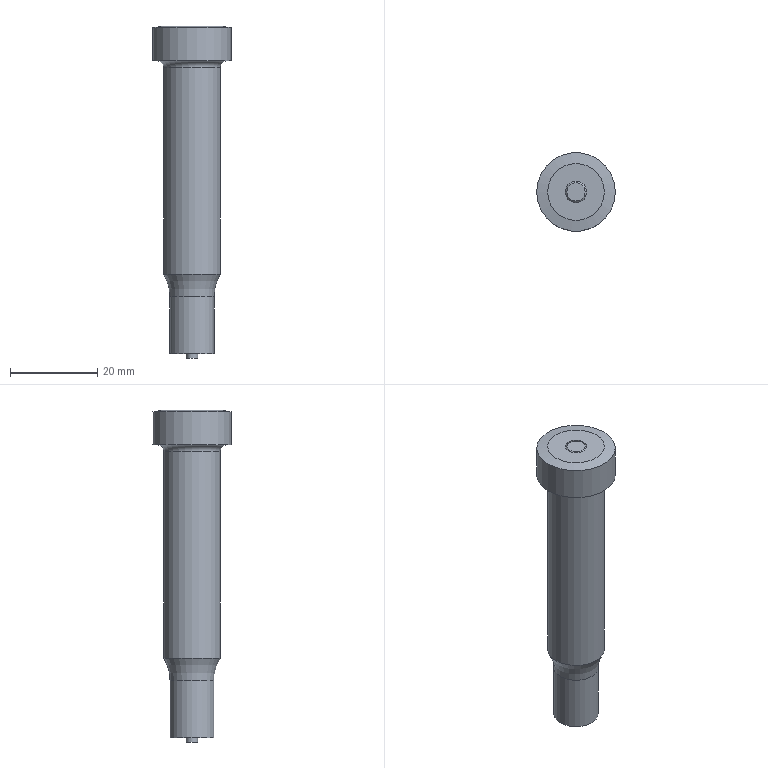Part | NX | features APJAS13-90-P10.10_2 2 | 1 solid | 20 faces | box 18 x 18 x 76 mm | volume 9972 mm3 | cylinder 8 | plane 7 | torus 2 | cone 2 | spline 1 | commonest cylinder face diameters 2.6 x1 2.8 x1 4.2 x1 4.4 x1 4.9 x1 10.1 x1
STEP:
#1=CARTESIAN_POINT('',(-223.5,0.,13.186));
#2=VERTEX_POINT('',#1);
#3=CARTESIAN_POINT('',(-230.,0.,13.186));
#4=DIRECTION('',(0.,0.,1.));
#5=DIRECTION('',(-1.,0.,0.));
#6=AXIS2_PLACEMENT_3D('',#3,#4,#5);
#7=CIRCLE('',#6,6.5);
#8=EDGE_CURVE('',#2,#2,#7,.T.);
#9=ORIENTED_EDGE('',*,*,#8,.T.);
#10=EDGE_LOOP('',(#9));
#11=FACE_BOUND('',#10,.T.);
#12=CARTESIAN_POINT('',(-236.5,0.,60.5));
#13=VERTEX_POINT('',#12);
#14=CARTESIAN_POINT('',(-230.,0.,60.5));
#15=DIRECTION('',(0.,0.,1.));
#16=DIRECTION('',(1.,0.,0.));
#17=AXIS2_PLACEMENT_3D('',#14,#15,#16);
#18=CIRCLE('',#17,6.5);
#19=EDGE_CURVE('',#13,#13,#18,.T.);
#20=ORIENTED_EDGE('',*,*,#19,.F.);
#21=EDGE_LOOP('',(#20));
#22=FACE_BOUND('',#21,.T.);
#23=CARTESIAN_POINT('',(-230.,0.,42.5));
#24=DIRECTION('',(0.,0.,-1.));
#25=DIRECTION('',(1.,0.,0.));
#26=AXIS2_PLACEMENT_3D('',#23,#24,#25);
#27=CYLINDRICAL_SURFACE('',#26,6.5);
#28=ADVANCED_FACE('',(#11,#22),#27,.T.);
#29=CARTESIAN_POINT('',(-231.4,0.,23.));
#30=VERTEX_POINT('',#29);
#31=CARTESIAN_POINT('',(-230.,0.,23.));
#32=DIRECTION('',(0.,0.,1.));
#33=DIRECTION('',(-1.,0.,0.));
#34=AXIS2_PLACEMENT_3D('',#31,#32,#33);
#35=CIRCLE('',#34,1.4);
#36=EDGE_CURVE('',#30,#30,#35,.T.);
#37=ORIENTED_EDGE('',*,*,#36,.T.);
#38=EDGE_LOOP('',(#37));
#39=FACE_BOUND('',#38,.T.);
#40=CARTESIAN_POINT('',(-231.4,0.,-5.));
#41=VERTEX_POINT('',#40);
#42=CARTESIAN_POINT('',(-230.,0.,-5.));
#43=DIRECTION('',(0.,0.,1.));
#44=DIRECTION('',(-1.,0.,0.));
#45=AXIS2_PLACEMENT_3D('',#42,#43,#44);
#46=CIRCLE('',#45,1.4);
#47=EDGE_CURVE('',#41,#41,#46,.T.);
#48=ORIENTED_EDGE('',*,*,#47,.F.);
#49=EDGE_LOOP('',(#48));
#50=FACE_BOUND('',#49,.T.);
#51=CARTESIAN_POINT('',(-230.,0.,9.));
#52=DIRECTION('',(0.,0.,-1.));
#53=DIRECTION('',(1.,0.,0.));
#54=AXIS2_PLACEMENT_3D('',#51,#52,#53);
#55=CYLINDRICAL_SURFACE('',#54,1.4);
#56=ADVANCED_FACE('',(#39,#50),#55,.F.);
#57=CARTESIAN_POINT('',(-227.55,0.,69.632));
#58=VERTEX_POINT('',#57);
#59=CARTESIAN_POINT('',(-230.,0.,69.632));
#60=DIRECTION('',(0.,0.,1.));
#61=DIRECTION('',(1.,0.,0.));
#62=AXIS2_PLACEMENT_3D('',#59,#60,#61);
#63=CIRCLE('',#62,2.45);
#64=EDGE_CURVE('',#58,#58,#63,.T.);
#65=ORIENTED_EDGE('',*,*,#64,.F.);
#66=EDGE_LOOP('',(#65));
#67=FACE_BOUND('',#66,.T.);
#68=CARTESIAN_POINT('',(-232.45,0.,70.));
#69=VERTEX_POINT('',#68);
#70=CARTESIAN_POINT('',(-230.,0.,70.));
#71=DIRECTION('',(0.,0.,-1.));
#72=DIRECTION('',(-1.,0.,0.));
#73=AXIS2_PLACEMENT_3D('',#70,#71,#72);
#74=CIRCLE('',#73,2.45);
#75=EDGE_CURVE('',#69,#69,#74,.T.);
#76=ORIENTED_EDGE('',*,*,#75,.F.);
#77=EDGE_LOOP('',(#76));
#78=FACE_BOUND('',#77,.T.);
#79=CARTESIAN_POINT('',(-230.,0.,68.775));
#80=DIRECTION('',(0.,0.,-1.));
#81=DIRECTION('',(1.,0.,0.));
#82=AXIS2_PLACEMENT_3D('',#79,#80,#81);
#83=CYLINDRICAL_SURFACE('',#82,2.45);
#84=ADVANCED_FACE('',(#67,#78),#83,.F.);
#85=ORIENTED_EDGE('',*,*,#19,.T.);
#86=EDGE_LOOP('',(#85));
#87=FACE_BOUND('',#86,.T.);
#88=CARTESIAN_POINT('',(-238.,0.,62.));
#89=VERTEX_POINT('',#88);
#90=CARTESIAN_POINT('',(-230.,0.,62.));
#91=DIRECTION('',(0.,0.,-1.));
#92=DIRECTION('',(1.,0.,0.));
#93=AXIS2_PLACEMENT_3D('',#90,#91,#92);
#94=CIRCLE('',#93,8.);
#95=EDGE_CURVE('',#89,#89,#94,.T.);
#96=ORIENTED_EDGE('',*,*,#95,.T.);
#97=EDGE_LOOP('',(#96));
#98=FACE_BOUND('',#97,.T.);
#99=CARTESIAN_POINT('',(-230.,0.,60.5));
#100=DIRECTION('',(0.,0.,1.));
#101=DIRECTION('',(-1.,0.,0.));
#102=AXIS2_PLACEMENT_3D('',#99,#100,#101);
#103=TOROIDAL_SURFACE('',#102,8.,1.5);
#104=ADVANCED_FACE('',(#87,#98),#103,.F.);
#105=CARTESIAN_POINT('',(-239.,0.,62.));
#106=VERTEX_POINT('',#105);
#107=CARTESIAN_POINT('',(-230.,0.,62.));
#108=DIRECTION('',(0.,0.,-1.));
#109=DIRECTION('',(-1.,0.,0.));
#110=AXIS2_PLACEMENT_3D('',#107,#108,#109);
#111=CIRCLE('',#110,9.);
#112=EDGE_CURVE('',#106,#106,#111,.T.);
#113=ORIENTED_EDGE('',*,*,#112,.T.);
#114=EDGE_LOOP('',(#113));
#115=FACE_BOUND('',#114,.T.);
#116=ORIENTED_EDGE('',*,*,#95,.F.);
#117=EDGE_LOOP('',(#116));
#118=FACE_BOUND('',#117,.T.);
#119=CARTESIAN_POINT('',(-230.,0.,62.));
#120=DIRECTION('',(0.,0.,-1.));
#121=DIRECTION('',(1.,0.,0.));
#122=AXIS2_PLACEMENT_3D('',#119,#120,#121);
#123=PLANE('',#122);
#124=ADVANCED_FACE('',(#115,#118),#123,.T.);
#125=CARTESIAN_POINT('',(-235.05,0.,8.));
#126=VERTEX_POINT('',#125);
#127=CARTESIAN_POINT('',(-230.,0.,8.));
#128=DIRECTION('',(0.,0.,1.));
#129=DIRECTION('',(-1.,0.,0.));
#130=AXIS2_PLACEMENT_3D('',#127,#128,#129);
#131=CIRCLE('',#130,5.05);
#132=EDGE_CURVE('',#126,#126,#131,.T.);
#133=ORIENTED_EDGE('',*,*,#132,.T.);
#134=EDGE_LOOP('',(#133));
#135=FACE_BOUND('',#134,.T.);
#136=ORIENTED_EDGE('',*,*,#8,.F.);
#137=EDGE_LOOP('',(#136));
#138=FACE_BOUND('',#137,.T.);
#139=CARTESIAN_POINT('',(-230.,0.,8.));
#140=DIRECTION('',(0.,0.,-1.));
#141=DIRECTION('',(1.,0.,0.));
#142=AXIS2_PLACEMENT_3D('',#139,#140,#141);
#143=TOROIDAL_SURFACE('',#142,15.05,10.);
#144=ADVANCED_FACE('',(#135,#138),#143,.F.);
#145=CARTESIAN_POINT('',(-239.,0.,69.559));
#146=VERTEX_POINT('',#145);
#147=CARTESIAN_POINT('',(-230.,0.,69.559));
#148=DIRECTION('',(0.,0.,1.));
#149=DIRECTION('',(1.,0.,0.));
#150=AXIS2_PLACEMENT_3D('',#147,#148,#149);
#151=CIRCLE('',#150,9.);
#152=EDGE_CURVE('',#146,#146,#151,.T.);
#153=ORIENTED_EDGE('',*,*,#152,.T.);
#154=EDGE_LOOP('',(#153));
#155=FACE_BOUND('',#154,.T.);
#156=CARTESIAN_POINT('',(-236.5,0.,70.));
#157=VERTEX_POINT('',#156);
#158=CARTESIAN_POINT('',(-230.,0.,70.));
#159=DIRECTION('',(0.,0.,-1.));
#160=DIRECTION('',(1.,0.,0.));
#161=AXIS2_PLACEMENT_3D('',#158,#159,#160);
#162=CIRCLE('',#161,6.5);
#163=EDGE_CURVE('',#157,#157,#162,.T.);
#164=ORIENTED_EDGE('',*,*,#163,.T.);
#165=EDGE_LOOP('',(#164));
#166=FACE_BOUND('',#165,.T.);
#167=CARTESIAN_POINT('',(-230.,0.,70.));
#168=DIRECTION('',(0.,0.,-1.));
#169=DIRECTION('',(-1.,0.,0.));
#170=AXIS2_PLACEMENT_3D('',#167,#168,#169);
#171=CONICAL_SURFACE('',#170,6.5,1.396);
#172=ADVANCED_FACE('',(#155,#166),#171,.T.);
#173=ORIENTED_EDGE('',*,*,#112,.F.);
#174=EDGE_LOOP('',(#173));
#175=FACE_BOUND('',#174,.T.);
#176=ORIENTED_EDGE('',*,*,#152,.F.);
#177=EDGE_LOOP('',(#176));
#178=FACE_BOUND('',#177,.T.);
#179=CARTESIAN_POINT('',(-230.,0.,66.));
#180=DIRECTION('',(0.,0.,-1.));
#181=DIRECTION('',(1.,0.,0.));
#182=AXIS2_PLACEMENT_3D('',#179,#180,#181);
#183=CYLINDRICAL_SURFACE('',#182,9.);
#184=ADVANCED_FACE('',(#175,#178),#183,.T.);
#185=ORIENTED_EDGE('',*,*,#75,.T.);
#186=EDGE_LOOP('',(#185));
#187=FACE_BOUND('',#186,.T.);
#188=ORIENTED_EDGE('',*,*,#163,.F.);
#189=EDGE_LOOP('',(#188));
#190=FACE_BOUND('',#189,.T.);
#191=CARTESIAN_POINT('',(-230.,0.,70.));
#192=DIRECTION('',(0.,0.,1.));
#193=DIRECTION('',(-1.,0.,0.));
#194=AXIS2_PLACEMENT_3D('',#191,#192,#193);
#195=PLANE('',#194);
#196=ADVANCED_FACE('',(#187,#190),#195,.T.);
#197=ORIENTED_EDGE('',*,*,#132,.F.);
#198=EDGE_LOOP('',(#197));
#199=FACE_BOUND('',#198,.T.);
#200=CARTESIAN_POINT('',(-235.05,0.,-5.));
#201=VERTEX_POINT('',#200);
#202=CARTESIAN_POINT('',(-230.,0.,-5.));
#203=DIRECTION('',(0.,0.,-1.));
#204=DIRECTION('',(-1.,0.,0.));
#205=AXIS2_PLACEMENT_3D('',#202,#203,#204);
#206=CIRCLE('',#205,5.05);
#207=EDGE_CURVE('',#201,#201,#206,.T.);
#208=ORIENTED_EDGE('',*,*,#207,.F.);
#209=EDGE_LOOP('',(#208));
#210=FACE_BOUND('',#209,.T.);
#211=CARTESIAN_POINT('',(-230.,0.,1.5));
#212=DIRECTION('',(0.,0.,-1.));
#213=DIRECTION('',(1.,0.,0.));
#214=AXIS2_PLACEMENT_3D('',#211,#212,#213);
#215=CYLINDRICAL_SURFACE('',#214,5.05);
#216=ADVANCED_FACE('',(#199,#210),#215,.T.);
#217=ORIENTED_EDGE('',*,*,#47,.T.);
#218=EDGE_LOOP('',(#217));
#219=FACE_BOUND('',#218,.T.);
#220=ORIENTED_EDGE('',*,*,#207,.T.);
#221=EDGE_LOOP('',(#220));
#222=FACE_BOUND('',#221,.T.);
#223=CARTESIAN_POINT('',(-230.,0.,-5.));
#224=DIRECTION('',(0.,0.,-1.));
#225=DIRECTION('',(1.,0.,0.));
#226=AXIS2_PLACEMENT_3D('',#223,#224,#225);
#227=PLANE('',#226);
#228=ADVANCED_FACE('',(#219,#222),#227,.T.);
#229=CARTESIAN_POINT('',(-227.917,0.,70.));
#230=VERTEX_POINT('',#229);
#231=CARTESIAN_POINT('',(-230.,0.,70.));
#232=DIRECTION('',(0.,0.,-1.));
#233=DIRECTION('',(1.,0.,0.));
#234=AXIS2_PLACEMENT_3D('',#231,#232,#233);
#235=CIRCLE('',#234,2.083);
#236=EDGE_CURVE('',#230,#230,#235,.T.);
#237=ORIENTED_EDGE('',*,*,#236,.F.);
#238=EDGE_LOOP('',(#237));
#239=FACE_BOUND('',#238,.T.);
#240=CARTESIAN_POINT('',(-230.,0.,70.));
#241=DIRECTION('',(0.,0.,1.));
#242=DIRECTION('',(-1.,0.,0.));
#243=AXIS2_PLACEMENT_3D('',#240,#241,#242);
#244=PLANE('',#243);
#245=ADVANCED_FACE('',(#239),#244,.T.);
#246=ORIENTED_EDGE('',*,*,#64,.T.);
#247=EDGE_LOOP('',(#246));
#248=FACE_BOUND('',#247,.T.);
#249=ORIENTED_EDGE('',*,*,#236,.T.);
#250=EDGE_LOOP('',(#249));
#251=FACE_BOUND('',#250,.T.);
#252=CARTESIAN_POINT('',(-230.,0.,70.));
#253=DIRECTION('',(0.,0.,-1.));
#254=DIRECTION('',(-1.,0.,0.));
#255=AXIS2_PLACEMENT_3D('',#252,#253,#254);
#256=CONICAL_SURFACE('',#255,2.083,0.7854);
#257=ADVANCED_FACE('',(#248,#251),#256,.T.);
#258=CARTESIAN_POINT('',(-231.3,0.,23.));
#259=VERTEX_POINT('',#258);
#260=CARTESIAN_POINT('',(-230.,0.,23.));
#261=DIRECTION('',(0.,0.,-1.));
#262=DIRECTION('',(-1.,0.,0.));
#263=AXIS2_PLACEMENT_3D('',#260,#261,#262);
#264=CIRCLE('',#263,1.3);
#265=EDGE_CURVE('',#259,#259,#264,.F.);
#266=ORIENTED_EDGE('',*,*,#265,.T.);
#267=EDGE_LOOP('',(#266));
#268=FACE_BOUND('',#267,.T.);
#269=ORIENTED_EDGE('',*,*,#36,.F.);
#270=EDGE_LOOP('',(#269));
#271=FACE_BOUND('',#270,.T.);
#272=CARTESIAN_POINT('',(-230.,0.,23.));
#273=DIRECTION('',(0.,0.,-1.));
#274=DIRECTION('',(1.,0.,0.));
#275=AXIS2_PLACEMENT_3D('',#272,#273,#274);
#276=PLANE('',#275);
#277=ADVANCED_FACE('',(#268,#271),#276,.T.);
#278=ORIENTED_EDGE('',*,*,#265,.F.);
#279=EDGE_LOOP('',(#278));
#280=FACE_BOUND('',#279,.T.);
#281=CARTESIAN_POINT('',(-231.3,0.,-6.));
#282=VERTEX_POINT('',#281);
#283=CARTESIAN_POINT('',(-230.,0.,-6.));
#284=DIRECTION('',(0.,0.,-1.));
#285=DIRECTION('',(-1.,0.,0.));
#286=AXIS2_PLACEMENT_3D('',#283,#284,#285);
#287=CIRCLE('',#286,1.3);
#288=EDGE_CURVE('',#282,#282,#287,.T.);
#289=ORIENTED_EDGE('',*,*,#288,.F.);
#290=EDGE_LOOP('',(#289));
#291=FACE_BOUND('',#290,.T.);
#292=CARTESIAN_POINT('',(-230.,0.,8.5));
#293=DIRECTION('',(0.,0.,-1.));
#294=DIRECTION('',(1.,0.,0.));
#295=AXIS2_PLACEMENT_3D('',#292,#293,#294);
#296=CYLINDRICAL_SURFACE('',#295,1.3);
#297=ADVANCED_FACE('',(#280,#291),#296,.T.);
#298=ORIENTED_EDGE('',*,*,#288,.T.);
#299=EDGE_LOOP('',(#298));
#300=FACE_BOUND('',#299,.T.);
#301=CARTESIAN_POINT('',(-230.,0.,-6.));
#302=DIRECTION('',(0.,0.,-1.));
#303=DIRECTION('',(1.,0.,0.));
#304=AXIS2_PLACEMENT_3D('',#301,#302,#303);
#305=PLANE('',#304);
#306=ADVANCED_FACE('',(#300),#305,.T.);
#307=CLOSED_SHELL('',(#28,#56,#84,#104,#124,#144,#172,#184,#196,#216,#228,#245,#257,#277,#297,#306));
#308=CARTESIAN_POINT('',(-227.8,0.001782,65.1));
#309=VERTEX_POINT('',#308);
#310=CARTESIAN_POINT('',(-228.276,-1.724,65.1));
#311=CARTESIAN_POINT('',(-227.561,0.00202,65.1));
#312=CARTESIAN_POINT('',(-228.279,1.727,65.1));
#313=CARTESIAN_POINT('',(-230.001,2.438,65.1));
#314=CARTESIAN_POINT('',(-231.727,1.722,65.1));
#315=CARTESIAN_POINT('',(-232.437,-0.001955,65.1));
#316=CARTESIAN_POINT('',(-231.724,-1.724,65.1));
#317=CARTESIAN_POINT('',(-229.998,-2.438,65.1));
#318=CARTESIAN_POINT('',(-228.276,-1.724,65.1));
#319=CARTESIAN_POINT('',(-227.561,0.00202,65.1));
#320=CARTESIAN_POINT('',(-228.279,1.727,65.1));
#321=B_SPLINE_CURVE_WITH_KNOTS('',3,(#310,#311,#312,#313,#314,#315,#316,#317,#318,#319,#320),.UNSPECIFIED.,.T.,.F.,(1,1,1,1,1,1,1,1,1,1,1,1,1,1,1),(-0.00518,-0.003453,-0.001727,0.,0.001727,0.003453,0.00518,0.006907,0.008633,0.01036,0.01209,0.01381,0.01554,0.01727,0.01899),.UNSPECIFIED.);
#322=EDGE_CURVE('',#309,#309,#321,.T.);
#323=ORIENTED_EDGE('',*,*,#322,.T.);
#324=EDGE_LOOP('',(#323));
#325=FACE_BOUND('',#324,.T.);
#326=CARTESIAN_POINT('',(-232.2,0.,23.));
#327=VERTEX_POINT('',#326);
#328=CARTESIAN_POINT('',(-230.,0.,23.));
#329=DIRECTION('',(0.,0.,-1.));
#330=DIRECTION('',(-1.,0.,0.));
#331=AXIS2_PLACEMENT_3D('',#328,#329,#330);
#332=CIRCLE('',#331,2.2);
#333=EDGE_CURVE('',#327,#327,#332,.T.);
#334=ORIENTED_EDGE('',*,*,#333,.T.);
#335=EDGE_LOOP('',(#334));
#336=FACE_BOUND('',#335,.T.);
#337=CARTESIAN_POINT('',(-230.,0.,52.775));
#338=DIRECTION('',(0.,0.,-1.));
#339=DIRECTION('',(1.,0.,0.));
#340=AXIS2_PLACEMENT_3D('',#337,#338,#339);
#341=CYLINDRICAL_SURFACE('',#340,2.2);
#342=ADVANCED_FACE('',(#325,#336),#341,.F.);
#343=CARTESIAN_POINT('',(-232.1,0.,23.));
#344=VERTEX_POINT('',#343);
#345=CARTESIAN_POINT('',(-230.,0.,23.));
#346=DIRECTION('',(0.,0.,-1.));
#347=DIRECTION('',(-1.,0.,0.));
#348=AXIS2_PLACEMENT_3D('',#345,#346,#347);
#349=CIRCLE('',#348,2.1);
#350=EDGE_CURVE('',#344,#344,#349,.T.);
#351=ORIENTED_EDGE('',*,*,#350,.T.);
#352=EDGE_LOOP('',(#351));
#353=FACE_BOUND('',#352,.T.);
#354=ORIENTED_EDGE('',*,*,#333,.F.);
#355=EDGE_LOOP('',(#354));
#356=FACE_BOUND('',#355,.T.);
#357=CARTESIAN_POINT('',(-230.,0.,23.));
#358=DIRECTION('',(0.,0.,-1.));
#359=DIRECTION('',(1.,0.,0.));
#360=AXIS2_PLACEMENT_3D('',#357,#358,#359);
#361=PLANE('',#360);
#362=ADVANCED_FACE('',(#353,#356),#361,.F.);
#363=ORIENTED_EDGE('',*,*,#322,.F.);
#364=CARTESIAN_POINT('',(-227.9,0.001701,64.961));
#365=VERTEX_POINT('',#364);
#366=CARTESIAN_POINT('',(-227.55,0.001984,65.448));
#367=DIRECTION('',(-0.5832,-0.0004724,-0.8123));
#368=VECTOR('',#367,1000.);
#369=LINE('',#366,#368);
#370=EDGE_CURVE('',#309,#365,#369,.T.);
#371=ORIENTED_EDGE('',*,*,#370,.T.);
#372=CARTESIAN_POINT('',(-227.9,0.,64.961));
#373=VERTEX_POINT('',#372);
#374=CARTESIAN_POINT('',(-227.9,0.001701,64.961));
#375=CARTESIAN_POINT('',(-227.9,0.5565,64.961));
#376=CARTESIAN_POINT('',(-228.357,1.645,64.961));
#377=CARTESIAN_POINT('',(-230.001,2.328,64.961));
#378=CARTESIAN_POINT('',(-231.647,1.644,64.961));
#379=CARTESIAN_POINT('',(-232.326,-0.000902,64.961));
#380=CARTESIAN_POINT('',(-231.647,-1.644,64.961));
#381=CARTESIAN_POINT('',(-230.,-2.328,64.961));
#382=CARTESIAN_POINT('',(-228.356,-1.644,64.961));
#383=CARTESIAN_POINT('',(-227.9,-0.5548,64.961));
#384=CARTESIAN_POINT('',(-227.9,0.,64.961));
#385=B_SPLINE_CURVE_WITH_KNOTS('',3,(#374,#375,#376,#377,#378,#379,#380,#381,#382,#383,#384),.UNSPECIFIED.,.F.,.F.,(4,1,1,1,1,1,1,1,4),(0.,0.001646,0.003293,0.004939,0.006585,0.008232,0.009878,0.01152,0.01317),.UNSPECIFIED.);
#386=EDGE_CURVE('',#365,#373,#385,.T.);
#387=ORIENTED_EDGE('',*,*,#386,.T.);
#388=CARTESIAN_POINT('',(-227.9,0.,64.961));
#389=CARTESIAN_POINT('',(-227.9,0.0005669,64.961));
#390=CARTESIAN_POINT('',(-227.9,0.001134,64.961));
#391=CARTESIAN_POINT('',(-227.9,0.001701,64.961));
#392=B_SPLINE_CURVE_WITH_KNOTS('',3,(#388,#389,#390,#391),.UNSPECIFIED.,.F.,.F.,(4,4),(0.003447,0.003449),.UNSPECIFIED.);
#393=EDGE_CURVE('',#373,#365,#392,.T.);
#394=ORIENTED_EDGE('',*,*,#393,.T.);
#395=ORIENTED_EDGE('',*,*,#370,.F.);
#396=EDGE_LOOP('',(#363,#371,#387,#394,#395));
#397=FACE_BOUND('',#396,.T.);
#398=CARTESIAN_POINT('',(-227.901,-0.2708,64.96));
#399=CARTESIAN_POINT('',(-227.901,-0.2708,64.96));
#400=CARTESIAN_POINT('',(-227.9,-0.2708,64.96));
#401=CARTESIAN_POINT('',(-227.9,-0.2709,64.961));
#402=CARTESIAN_POINT('',(-227.867,-0.2751,65.006));
#403=CARTESIAN_POINT('',(-227.835,-0.2793,65.051));
#404=CARTESIAN_POINT('',(-227.803,-0.2834,65.097));
#405=CARTESIAN_POINT('',(-227.802,-0.2836,65.098));
#406=CARTESIAN_POINT('',(-227.801,-0.2837,65.099));
#407=CARTESIAN_POINT('',(-227.8,-0.2838,65.1));
#408=CARTESIAN_POINT('',(-227.8,-0.2838,65.101));
#409=CARTESIAN_POINT('',(-227.799,-0.2839,65.101));
#410=CARTESIAN_POINT('',(-227.799,-0.2839,65.102));
#411=CARTESIAN_POINT('',(-227.901,0.1543,64.96));
#412=CARTESIAN_POINT('',(-227.901,0.1543,64.96));
#413=CARTESIAN_POINT('',(-227.9,0.1543,64.96));
#414=CARTESIAN_POINT('',(-227.9,0.1544,64.961));
#415=CARTESIAN_POINT('',(-227.867,0.1567,65.006));
#416=CARTESIAN_POINT('',(-227.835,0.1591,65.051));
#417=CARTESIAN_POINT('',(-227.803,0.1615,65.097));
#418=CARTESIAN_POINT('',(-227.802,0.1616,65.098));
#419=CARTESIAN_POINT('',(-227.801,0.1616,65.099));
#420=CARTESIAN_POINT('',(-227.8,0.1617,65.1));
#421=CARTESIAN_POINT('',(-227.8,0.1617,65.101));
#422=CARTESIAN_POINT('',(-227.799,0.1618,65.101));
#423=CARTESIAN_POINT('',(-227.799,0.1618,65.102));
#424=CARTESIAN_POINT('',(-227.918,0.3095,64.96));
#425=CARTESIAN_POINT('',(-227.918,0.3096,64.96));
#426=CARTESIAN_POINT('',(-227.917,0.3096,64.96));
#427=CARTESIAN_POINT('',(-227.917,0.3096,64.961));
#428=CARTESIAN_POINT('',(-227.885,0.3144,65.006));
#429=CARTESIAN_POINT('',(-227.853,0.3192,65.051));
#430=CARTESIAN_POINT('',(-227.821,0.324,65.097));
#431=CARTESIAN_POINT('',(-227.82,0.3241,65.098));
#432=CARTESIAN_POINT('',(-227.819,0.3243,65.099));
#433=CARTESIAN_POINT('',(-227.818,0.3244,65.1));
#434=CARTESIAN_POINT('',(-227.818,0.3244,65.101));
#435=CARTESIAN_POINT('',(-227.817,0.3245,65.101));
#436=CARTESIAN_POINT('',(-227.817,0.3246,65.102));
#437=CARTESIAN_POINT('',(-227.986,0.6106,64.96));
#438=CARTESIAN_POINT('',(-227.985,0.6107,64.96));
#439=CARTESIAN_POINT('',(-227.985,0.6108,64.96));
#440=CARTESIAN_POINT('',(-227.985,0.6108,64.961));
#441=CARTESIAN_POINT('',(-227.954,0.6203,65.006));
#442=CARTESIAN_POINT('',(-227.923,0.6297,65.051));
#443=CARTESIAN_POINT('',(-227.891,0.6392,65.097));
#444=CARTESIAN_POINT('',(-227.891,0.6394,65.098));
#445=CARTESIAN_POINT('',(-227.89,0.6397,65.099));
#446=CARTESIAN_POINT('',(-227.889,0.6399,65.1));
#447=CARTESIAN_POINT('',(-227.889,0.64,65.101));
#448=CARTESIAN_POINT('',(-227.888,0.6402,65.101));
#449=CARTESIAN_POINT('',(-227.888,0.6403,65.102));
#450=CARTESIAN_POINT('',(-228.036,0.7583,64.96));
#451=CARTESIAN_POINT('',(-228.036,0.7584,64.96));
#452=CARTESIAN_POINT('',(-228.036,0.7585,64.96));
#453=CARTESIAN_POINT('',(-228.036,0.7586,64.961));
#454=CARTESIAN_POINT('',(-228.005,0.7703,65.006));
#455=CARTESIAN_POINT('',(-227.975,0.7821,65.051));
#456=CARTESIAN_POINT('',(-227.945,0.7938,65.097));
#457=CARTESIAN_POINT('',(-227.944,0.7941,65.098));
#458=CARTESIAN_POINT('',(-227.943,0.7944,65.099));
#459=CARTESIAN_POINT('',(-227.942,0.7947,65.1));
#460=CARTESIAN_POINT('',(-227.942,0.7948,65.101));
#461=CARTESIAN_POINT('',(-227.941,0.795,65.101));
#462=CARTESIAN_POINT('',(-227.941,0.7951,65.102));
#463=CARTESIAN_POINT('',(-228.218,1.143,64.96));
#464=CARTESIAN_POINT('',(-228.218,1.143,64.96));
#465=CARTESIAN_POINT('',(-228.218,1.143,64.96));
#466=CARTESIAN_POINT('',(-228.218,1.143,64.961));
#467=CARTESIAN_POINT('',(-228.19,1.161,65.006));
#468=CARTESIAN_POINT('',(-228.162,1.178,65.051));
#469=CARTESIAN_POINT('',(-228.135,1.196,65.097));
#470=CARTESIAN_POINT('',(-228.134,1.196,65.098));
#471=CARTESIAN_POINT('',(-228.133,1.197,65.099));
#472=CARTESIAN_POINT('',(-228.133,1.197,65.1));
#473=CARTESIAN_POINT('',(-228.132,1.198,65.101));
#474=CARTESIAN_POINT('',(-228.132,1.198,65.101));
#475=CARTESIAN_POINT('',(-228.132,1.198,65.102));
#476=CARTESIAN_POINT('',(-228.385,1.368,64.96));
#477=CARTESIAN_POINT('',(-228.385,1.369,64.96));
#478=CARTESIAN_POINT('',(-228.385,1.369,64.96));
#479=CARTESIAN_POINT('',(-228.385,1.369,64.961));
#480=CARTESIAN_POINT('',(-228.36,1.39,65.006));
#481=CARTESIAN_POINT('',(-228.335,1.411,65.051));
#482=CARTESIAN_POINT('',(-228.31,1.433,65.097));
#483=CARTESIAN_POINT('',(-228.309,1.433,65.098));
#484=CARTESIAN_POINT('',(-228.308,1.434,65.099));
#485=CARTESIAN_POINT('',(-228.308,1.434,65.1));
#486=CARTESIAN_POINT('',(-228.307,1.434,65.101));
#487=CARTESIAN_POINT('',(-228.307,1.435,65.101));
#488=CARTESIAN_POINT('',(-228.307,1.435,65.102));
#489=CARTESIAN_POINT('',(-228.785,1.733,64.96));
#490=CARTESIAN_POINT('',(-228.785,1.734,64.96));
#491=CARTESIAN_POINT('',(-228.785,1.734,64.96));
#492=CARTESIAN_POINT('',(-228.785,1.734,64.961));
#493=CARTESIAN_POINT('',(-228.766,1.761,65.006));
#494=CARTESIAN_POINT('',(-228.747,1.788,65.051));
#495=CARTESIAN_POINT('',(-228.729,1.815,65.097));
#496=CARTESIAN_POINT('',(-228.728,1.815,65.098));
#497=CARTESIAN_POINT('',(-228.728,1.816,65.099));
#498=CARTESIAN_POINT('',(-228.727,1.817,65.1));
#499=CARTESIAN_POINT('',(-228.727,1.817,65.101));
#500=CARTESIAN_POINT('',(-228.727,1.817,65.101));
#501=CARTESIAN_POINT('',(-228.726,1.818,65.102));
#502=CARTESIAN_POINT('',(-229.026,1.879,64.96));
#503=CARTESIAN_POINT('',(-229.026,1.879,64.96));
#504=CARTESIAN_POINT('',(-229.025,1.88,64.96));
#505=CARTESIAN_POINT('',(-229.025,1.88,64.961));
#506=CARTESIAN_POINT('',(-229.01,1.909,65.006));
#507=CARTESIAN_POINT('',(-228.995,1.938,65.051));
#508=CARTESIAN_POINT('',(-228.98,1.967,65.097));
#509=CARTESIAN_POINT('',(-228.98,1.968,65.098));
#510=CARTESIAN_POINT('',(-228.979,1.969,65.099));
#511=CARTESIAN_POINT('',(-228.979,1.969,65.1));
#512=CARTESIAN_POINT('',(-228.979,1.97,65.101));
#513=CARTESIAN_POINT('',(-228.979,1.97,65.101));
#514=CARTESIAN_POINT('',(-228.978,1.97,65.102));
#515=CARTESIAN_POINT('',(-229.534,2.065,64.96));
#516=CARTESIAN_POINT('',(-229.534,2.065,64.96));
#517=CARTESIAN_POINT('',(-229.534,2.065,64.96));
#518=CARTESIAN_POINT('',(-229.534,2.066,64.961));
#519=CARTESIAN_POINT('',(-229.527,2.098,65.006));
#520=CARTESIAN_POINT('',(-229.52,2.129,65.051));
#521=CARTESIAN_POINT('',(-229.513,2.161,65.097));
#522=CARTESIAN_POINT('',(-229.512,2.162,65.098));
#523=CARTESIAN_POINT('',(-229.512,2.163,65.099));
#524=CARTESIAN_POINT('',(-229.512,2.164,65.1));
#525=CARTESIAN_POINT('',(-229.512,2.164,65.101));
#526=CARTESIAN_POINT('',(-229.512,2.165,65.101));
#527=CARTESIAN_POINT('',(-229.512,2.165,65.102));
#528=CARTESIAN_POINT('',(-229.812,2.108,64.96));
#529=CARTESIAN_POINT('',(-229.812,2.108,64.96));
#530=CARTESIAN_POINT('',(-229.812,2.109,64.96));
#531=CARTESIAN_POINT('',(-229.812,2.109,64.961));
#532=CARTESIAN_POINT('',(-229.809,2.142,65.006));
#533=CARTESIAN_POINT('',(-229.806,2.174,65.051));
#534=CARTESIAN_POINT('',(-229.803,2.207,65.097));
#535=CARTESIAN_POINT('',(-229.803,2.208,65.098));
#536=CARTESIAN_POINT('',(-229.803,2.209,65.099));
#537=CARTESIAN_POINT('',(-229.803,2.209,65.1));
#538=CARTESIAN_POINT('',(-229.803,2.21,65.101));
#539=CARTESIAN_POINT('',(-229.803,2.21,65.101));
#540=CARTESIAN_POINT('',(-229.803,2.211,65.102));
#541=CARTESIAN_POINT('',(-230.353,2.087,64.96));
#542=CARTESIAN_POINT('',(-230.353,2.087,64.96));
#543=CARTESIAN_POINT('',(-230.353,2.087,64.96));
#544=CARTESIAN_POINT('',(-230.353,2.088,64.961));
#545=CARTESIAN_POINT('',(-230.359,2.12,65.006));
#546=CARTESIAN_POINT('',(-230.364,2.152,65.051));
#547=CARTESIAN_POINT('',(-230.37,2.185,65.097));
#548=CARTESIAN_POINT('',(-230.37,2.185,65.098));
#549=CARTESIAN_POINT('',(-230.37,2.186,65.099));
#550=CARTESIAN_POINT('',(-230.37,2.187,65.1));
#551=CARTESIAN_POINT('',(-230.37,2.188,65.101));
#552=CARTESIAN_POINT('',(-230.37,2.188,65.101));
#553=CARTESIAN_POINT('',(-230.37,2.188,65.102));
#554=CARTESIAN_POINT('',(-230.627,2.022,64.96));
#555=CARTESIAN_POINT('',(-230.627,2.022,64.96));
#556=CARTESIAN_POINT('',(-230.627,2.022,64.96));
#557=CARTESIAN_POINT('',(-230.627,2.023,64.961));
#558=CARTESIAN_POINT('',(-230.636,2.054,65.006));
#559=CARTESIAN_POINT('',(-230.646,2.085,65.051));
#560=CARTESIAN_POINT('',(-230.656,2.116,65.097));
#561=CARTESIAN_POINT('',(-230.656,2.117,65.098));
#562=CARTESIAN_POINT('',(-230.656,2.118,65.099));
#563=CARTESIAN_POINT('',(-230.657,2.119,65.1));
#564=CARTESIAN_POINT('',(-230.657,2.119,65.101));
#565=CARTESIAN_POINT('',(-230.657,2.12,65.101));
#566=CARTESIAN_POINT('',(-230.657,2.12,65.102));
#567=CARTESIAN_POINT('',(-231.119,1.797,64.96));
#568=CARTESIAN_POINT('',(-231.119,1.797,64.96));
#569=CARTESIAN_POINT('',(-231.119,1.797,64.96));
#570=CARTESIAN_POINT('',(-231.119,1.797,64.961));
#571=CARTESIAN_POINT('',(-231.137,1.825,65.006));
#572=CARTESIAN_POINT('',(-231.154,1.853,65.051));
#573=CARTESIAN_POINT('',(-231.171,1.881,65.097));
#574=CARTESIAN_POINT('',(-231.172,1.881,65.098));
#575=CARTESIAN_POINT('',(-231.172,1.882,65.099));
#576=CARTESIAN_POINT('',(-231.173,1.883,65.1));
#577=CARTESIAN_POINT('',(-231.173,1.883,65.101));
#578=CARTESIAN_POINT('',(-231.173,1.884,65.101));
#579=CARTESIAN_POINT('',(-231.173,1.884,65.102));
#580=CARTESIAN_POINT('',(-231.347,1.633,64.96));
#581=CARTESIAN_POINT('',(-231.347,1.633,64.96));
#582=CARTESIAN_POINT('',(-231.348,1.633,64.96));
#583=CARTESIAN_POINT('',(-231.348,1.633,64.961));
#584=CARTESIAN_POINT('',(-231.369,1.658,65.006));
#585=CARTESIAN_POINT('',(-231.389,1.684,65.051));
#586=CARTESIAN_POINT('',(-231.41,1.709,65.097));
#587=CARTESIAN_POINT('',(-231.411,1.71,65.098));
#588=CARTESIAN_POINT('',(-231.411,1.71,65.099));
#589=CARTESIAN_POINT('',(-231.412,1.711,65.1));
#590=CARTESIAN_POINT('',(-231.412,1.711,65.101));
#591=CARTESIAN_POINT('',(-231.412,1.712,65.101));
#592=CARTESIAN_POINT('',(-231.413,1.712,65.102));
#593=CARTESIAN_POINT('',(-231.717,1.237,64.96));
#594=CARTESIAN_POINT('',(-231.718,1.237,64.96));
#595=CARTESIAN_POINT('',(-231.718,1.238,64.96));
#596=CARTESIAN_POINT('',(-231.718,1.238,64.961));
#597=CARTESIAN_POINT('',(-231.745,1.257,65.006));
#598=CARTESIAN_POINT('',(-231.771,1.276,65.051));
#599=CARTESIAN_POINT('',(-231.798,1.295,65.097));
#600=CARTESIAN_POINT('',(-231.798,1.296,65.098));
#601=CARTESIAN_POINT('',(-231.799,1.296,65.099));
#602=CARTESIAN_POINT('',(-231.8,1.297,65.1));
#603=CARTESIAN_POINT('',(-231.8,1.297,65.101));
#604=CARTESIAN_POINT('',(-231.8,1.297,65.101));
#605=CARTESIAN_POINT('',(-231.801,1.297,65.102));
#606=CARTESIAN_POINT('',(-231.866,0.9988,64.96));
#607=CARTESIAN_POINT('',(-231.866,0.999,64.96));
#608=CARTESIAN_POINT('',(-231.867,0.9991,64.96));
#609=CARTESIAN_POINT('',(-231.867,0.9992,64.961));
#610=CARTESIAN_POINT('',(-231.896,1.015,65.006));
#611=CARTESIAN_POINT('',(-231.925,1.03,65.051));
#612=CARTESIAN_POINT('',(-231.953,1.046,65.097));
#613=CARTESIAN_POINT('',(-231.954,1.046,65.098));
#614=CARTESIAN_POINT('',(-231.955,1.046,65.099));
#615=CARTESIAN_POINT('',(-231.956,1.047,65.1));
#616=CARTESIAN_POINT('',(-231.956,1.047,65.101));
#617=CARTESIAN_POINT('',(-231.956,1.047,65.101));
#618=CARTESIAN_POINT('',(-231.957,1.047,65.102));
#619=CARTESIAN_POINT('',(-232.058,0.4926,64.96));
#620=CARTESIAN_POINT('',(-232.059,0.4927,64.96));
#621=CARTESIAN_POINT('',(-232.059,0.4927,64.96));
#622=CARTESIAN_POINT('',(-232.059,0.4928,64.961));
#623=CARTESIAN_POINT('',(-232.091,0.5004,65.006));
#624=CARTESIAN_POINT('',(-232.123,0.5081,65.051));
#625=CARTESIAN_POINT('',(-232.155,0.5157,65.097));
#626=CARTESIAN_POINT('',(-232.156,0.5159,65.098));
#627=CARTESIAN_POINT('',(-232.156,0.5161,65.099));
#628=CARTESIAN_POINT('',(-232.157,0.5163,65.1));
#629=CARTESIAN_POINT('',(-232.158,0.5164,65.101));
#630=CARTESIAN_POINT('',(-232.158,0.5165,65.101));
#631=CARTESIAN_POINT('',(-232.158,0.5165,65.102));
#632=CARTESIAN_POINT('',(-232.106,0.2156,64.96));
#633=CARTESIAN_POINT('',(-232.106,0.2156,64.96));
#634=CARTESIAN_POINT('',(-232.106,0.2156,64.96));
#635=CARTESIAN_POINT('',(-232.106,0.2157,64.961));
#636=CARTESIAN_POINT('',(-232.139,0.219,65.006));
#637=CARTESIAN_POINT('',(-232.172,0.2223,65.051));
#638=CARTESIAN_POINT('',(-232.204,0.2257,65.097));
#639=CARTESIAN_POINT('',(-232.205,0.2258,65.098));
#640=CARTESIAN_POINT('',(-232.206,0.2259,65.099));
#641=CARTESIAN_POINT('',(-232.207,0.2259,65.1));
#642=CARTESIAN_POINT('',(-232.207,0.226,65.101));
#643=CARTESIAN_POINT('',(-232.207,0.226,65.101));
#644=CARTESIAN_POINT('',(-232.208,0.2261,65.102));
#645=CARTESIAN_POINT('',(-232.091,-0.3258,64.96));
#646=CARTESIAN_POINT('',(-232.092,-0.3258,64.96));
#647=CARTESIAN_POINT('',(-232.092,-0.3258,64.96));
#648=CARTESIAN_POINT('',(-232.092,-0.3259,64.961));
#649=CARTESIAN_POINT('',(-232.125,-0.3309,65.006));
#650=CARTESIAN_POINT('',(-232.157,-0.336,65.051));
#651=CARTESIAN_POINT('',(-232.189,-0.341,65.097));
#652=CARTESIAN_POINT('',(-232.19,-0.3412,65.098));
#653=CARTESIAN_POINT('',(-232.191,-0.3413,65.099));
#654=CARTESIAN_POINT('',(-232.192,-0.3414,65.1));
#655=CARTESIAN_POINT('',(-232.192,-0.3415,65.101));
#656=CARTESIAN_POINT('',(-232.193,-0.3415,65.101));
#657=CARTESIAN_POINT('',(-232.193,-0.3416,65.102));
#658=CARTESIAN_POINT('',(-232.03,-0.5999,64.96));
#659=CARTESIAN_POINT('',(-232.03,-0.6,64.96));
#660=CARTESIAN_POINT('',(-232.03,-0.6001,64.96));
#661=CARTESIAN_POINT('',(-232.031,-0.6002,64.961));
#662=CARTESIAN_POINT('',(-232.062,-0.6095,65.006));
#663=CARTESIAN_POINT('',(-232.093,-0.6187,65.051));
#664=CARTESIAN_POINT('',(-232.125,-0.628,65.097));
#665=CARTESIAN_POINT('',(-232.126,-0.6283,65.098));
#666=CARTESIAN_POINT('',(-232.126,-0.6285,65.099));
#667=CARTESIAN_POINT('',(-232.127,-0.6287,65.1));
#668=CARTESIAN_POINT('',(-232.128,-0.6289,65.101));
#669=CARTESIAN_POINT('',(-232.128,-0.629,65.101));
#670=CARTESIAN_POINT('',(-232.128,-0.6291,65.102));
#671=CARTESIAN_POINT('',(-231.811,-1.095,64.96));
#672=CARTESIAN_POINT('',(-231.811,-1.096,64.96));
#673=CARTESIAN_POINT('',(-231.812,-1.096,64.96));
#674=CARTESIAN_POINT('',(-231.812,-1.096,64.961));
#675=CARTESIAN_POINT('',(-231.84,-1.113,65.006));
#676=CARTESIAN_POINT('',(-231.868,-1.13,65.051));
#677=CARTESIAN_POINT('',(-231.896,-1.147,65.097));
#678=CARTESIAN_POINT('',(-231.897,-1.147,65.098));
#679=CARTESIAN_POINT('',(-231.897,-1.148,65.099));
#680=CARTESIAN_POINT('',(-231.898,-1.148,65.1));
#681=CARTESIAN_POINT('',(-231.898,-1.148,65.101));
#682=CARTESIAN_POINT('',(-231.899,-1.148,65.101));
#683=CARTESIAN_POINT('',(-231.899,-1.149,65.102));
#684=CARTESIAN_POINT('',(-231.65,-1.326,64.96));
#685=CARTESIAN_POINT('',(-231.65,-1.326,64.96));
#686=CARTESIAN_POINT('',(-231.65,-1.326,64.96));
#687=CARTESIAN_POINT('',(-231.651,-1.326,64.961));
#688=CARTESIAN_POINT('',(-231.676,-1.347,65.006));
#689=CARTESIAN_POINT('',(-231.702,-1.367,65.051));
#690=CARTESIAN_POINT('',(-231.727,-1.388,65.097));
#691=CARTESIAN_POINT('',(-231.728,-1.388,65.098));
#692=CARTESIAN_POINT('',(-231.729,-1.389,65.099));
#693=CARTESIAN_POINT('',(-231.729,-1.389,65.1));
#694=CARTESIAN_POINT('',(-231.73,-1.39,65.101));
#695=CARTESIAN_POINT('',(-231.73,-1.39,65.101));
#696=CARTESIAN_POINT('',(-231.73,-1.39,65.102));
#697=CARTESIAN_POINT('',(-231.26,-1.701,64.96));
#698=CARTESIAN_POINT('',(-231.26,-1.701,64.96));
#699=CARTESIAN_POINT('',(-231.26,-1.701,64.96));
#700=CARTESIAN_POINT('',(-231.26,-1.702,64.961));
#701=CARTESIAN_POINT('',(-231.28,-1.728,65.006));
#702=CARTESIAN_POINT('',(-231.299,-1.754,65.051));
#703=CARTESIAN_POINT('',(-231.319,-1.781,65.097));
#704=CARTESIAN_POINT('',(-231.319,-1.781,65.098));
#705=CARTESIAN_POINT('',(-231.32,-1.782,65.099));
#706=CARTESIAN_POINT('',(-231.32,-1.783,65.1));
#707=CARTESIAN_POINT('',(-231.32,-1.783,65.101));
#708=CARTESIAN_POINT('',(-231.321,-1.783,65.101));
#709=CARTESIAN_POINT('',(-231.321,-1.784,65.102));
#710=CARTESIAN_POINT('',(-231.023,-1.853,64.96));
#711=CARTESIAN_POINT('',(-231.023,-1.853,64.96));
#712=CARTESIAN_POINT('',(-231.023,-1.853,64.96));
#713=CARTESIAN_POINT('',(-231.024,-1.854,64.961));
#714=CARTESIAN_POINT('',(-231.039,-1.882,65.006));
#715=CARTESIAN_POINT('',(-231.055,-1.911,65.051));
#716=CARTESIAN_POINT('',(-231.071,-1.94,65.097));
#717=CARTESIAN_POINT('',(-231.072,-1.94,65.098));
#718=CARTESIAN_POINT('',(-231.072,-1.941,65.099));
#719=CARTESIAN_POINT('',(-231.072,-1.942,65.1));
#720=CARTESIAN_POINT('',(-231.073,-1.942,65.101));
#721=CARTESIAN_POINT('',(-231.073,-1.942,65.101));
#722=CARTESIAN_POINT('',(-231.073,-1.943,65.102));
#723=CARTESIAN_POINT('',(-230.52,-2.052,64.96));
#724=CARTESIAN_POINT('',(-230.52,-2.052,64.96));
#725=CARTESIAN_POINT('',(-230.52,-2.052,64.96));
#726=CARTESIAN_POINT('',(-230.52,-2.053,64.961));
#727=CARTESIAN_POINT('',(-230.528,-2.084,65.006));
#728=CARTESIAN_POINT('',(-230.536,-2.116,65.051));
#729=CARTESIAN_POINT('',(-230.544,-2.148,65.097));
#730=CARTESIAN_POINT('',(-230.544,-2.149,65.098));
#731=CARTESIAN_POINT('',(-230.544,-2.15,65.099));
#732=CARTESIAN_POINT('',(-230.545,-2.15,65.1));
#733=CARTESIAN_POINT('',(-230.545,-2.151,65.101));
#734=CARTESIAN_POINT('',(-230.545,-2.151,65.101));
#735=CARTESIAN_POINT('',(-230.545,-2.152,65.102));
#736=CARTESIAN_POINT('',(-230.243,-2.103,64.96));
#737=CARTESIAN_POINT('',(-230.243,-2.103,64.96));
#738=CARTESIAN_POINT('',(-230.243,-2.103,64.96));
#739=CARTESIAN_POINT('',(-230.243,-2.103,64.961));
#740=CARTESIAN_POINT('',(-230.247,-2.136,65.006));
#741=CARTESIAN_POINT('',(-230.251,-2.168,65.051));
#742=CARTESIAN_POINT('',(-230.255,-2.201,65.097));
#743=CARTESIAN_POINT('',(-230.255,-2.202,65.098));
#744=CARTESIAN_POINT('',(-230.255,-2.203,65.099));
#745=CARTESIAN_POINT('',(-230.255,-2.204,65.1));
#746=CARTESIAN_POINT('',(-230.255,-2.204,65.101));
#747=CARTESIAN_POINT('',(-230.255,-2.204,65.101));
#748=CARTESIAN_POINT('',(-230.255,-2.205,65.102));
#749=CARTESIAN_POINT('',(-229.702,-2.095,64.96));
#750=CARTESIAN_POINT('',(-229.702,-2.096,64.96));
#751=CARTESIAN_POINT('',(-229.702,-2.096,64.96));
#752=CARTESIAN_POINT('',(-229.702,-2.096,64.961));
#753=CARTESIAN_POINT('',(-229.697,-2.129,65.006));
#754=CARTESIAN_POINT('',(-229.692,-2.161,65.051));
#755=CARTESIAN_POINT('',(-229.688,-2.194,65.097));
#756=CARTESIAN_POINT('',(-229.688,-2.194,65.098));
#757=CARTESIAN_POINT('',(-229.688,-2.195,65.099));
#758=CARTESIAN_POINT('',(-229.687,-2.196,65.1));
#759=CARTESIAN_POINT('',(-229.687,-2.196,65.101));
#760=CARTESIAN_POINT('',(-229.687,-2.197,65.101));
#761=CARTESIAN_POINT('',(-229.687,-2.197,65.102));
#762=CARTESIAN_POINT('',(-229.427,-2.037,64.96));
#763=CARTESIAN_POINT('',(-229.427,-2.038,64.96));
#764=CARTESIAN_POINT('',(-229.427,-2.038,64.96));
#765=CARTESIAN_POINT('',(-229.427,-2.038,64.961));
#766=CARTESIAN_POINT('',(-229.418,-2.07,65.006));
#767=CARTESIAN_POINT('',(-229.409,-2.101,65.051));
#768=CARTESIAN_POINT('',(-229.4,-2.133,65.097));
#769=CARTESIAN_POINT('',(-229.4,-2.134,65.098));
#770=CARTESIAN_POINT('',(-229.399,-2.135,65.099));
#771=CARTESIAN_POINT('',(-229.399,-2.135,65.1));
#772=CARTESIAN_POINT('',(-229.399,-2.136,65.101));
#773=CARTESIAN_POINT('',(-229.399,-2.136,65.101));
#774=CARTESIAN_POINT('',(-229.399,-2.136,65.102));
#775=CARTESIAN_POINT('',(-228.929,-1.825,64.96));
#776=CARTESIAN_POINT('',(-228.928,-1.826,64.96));
#777=CARTESIAN_POINT('',(-228.928,-1.826,64.96));
#778=CARTESIAN_POINT('',(-228.928,-1.826,64.961));
#779=CARTESIAN_POINT('',(-228.911,-1.854,65.006));
#780=CARTESIAN_POINT('',(-228.895,-1.883,65.051));
#781=CARTESIAN_POINT('',(-228.878,-1.911,65.097));
#782=CARTESIAN_POINT('',(-228.878,-1.912,65.098));
#783=CARTESIAN_POINT('',(-228.877,-1.912,65.099));
#784=CARTESIAN_POINT('',(-228.877,-1.913,65.1));
#785=CARTESIAN_POINT('',(-228.877,-1.913,65.101));
#786=CARTESIAN_POINT('',(-228.877,-1.914,65.101));
#787=CARTESIAN_POINT('',(-228.876,-1.914,65.102));
#788=CARTESIAN_POINT('',(-228.696,-1.667,64.96));
#789=CARTESIAN_POINT('',(-228.696,-1.668,64.96));
#790=CARTESIAN_POINT('',(-228.696,-1.668,64.96));
#791=CARTESIAN_POINT('',(-228.696,-1.668,64.961));
#792=CARTESIAN_POINT('',(-228.675,-1.694,65.006));
#793=CARTESIAN_POINT('',(-228.655,-1.72,65.051));
#794=CARTESIAN_POINT('',(-228.635,-1.745,65.097));
#795=CARTESIAN_POINT('',(-228.635,-1.746,65.098));
#796=CARTESIAN_POINT('',(-228.634,-1.747,65.099));
#797=CARTESIAN_POINT('',(-228.634,-1.747,65.1));
#798=CARTESIAN_POINT('',(-228.633,-1.748,65.101));
#799=CARTESIAN_POINT('',(-228.633,-1.748,65.101));
#800=CARTESIAN_POINT('',(-228.633,-1.748,65.102));
#801=CARTESIAN_POINT('',(-228.316,-1.282,64.96));
#802=CARTESIAN_POINT('',(-228.316,-1.282,64.96));
#803=CARTESIAN_POINT('',(-228.315,-1.282,64.96));
#804=CARTESIAN_POINT('',(-228.315,-1.282,64.961));
#805=CARTESIAN_POINT('',(-228.289,-1.302,65.006));
#806=CARTESIAN_POINT('',(-228.263,-1.322,65.051));
#807=CARTESIAN_POINT('',(-228.237,-1.342,65.097));
#808=CARTESIAN_POINT('',(-228.236,-1.342,65.098));
#809=CARTESIAN_POINT('',(-228.236,-1.343,65.099));
#810=CARTESIAN_POINT('',(-228.235,-1.343,65.1));
#811=CARTESIAN_POINT('',(-228.235,-1.344,65.101));
#812=CARTESIAN_POINT('',(-228.234,-1.344,65.101));
#813=CARTESIAN_POINT('',(-228.234,-1.344,65.102));
#814=CARTESIAN_POINT('',(-228.161,-1.047,64.96));
#815=CARTESIAN_POINT('',(-228.161,-1.048,64.96));
#816=CARTESIAN_POINT('',(-228.16,-1.048,64.96));
#817=CARTESIAN_POINT('',(-228.16,-1.048,64.961));
#818=CARTESIAN_POINT('',(-228.132,-1.064,65.006));
#819=CARTESIAN_POINT('',(-228.103,-1.08,65.051));
#820=CARTESIAN_POINT('',(-228.075,-1.097,65.097));
#821=CARTESIAN_POINT('',(-228.074,-1.097,65.098));
#822=CARTESIAN_POINT('',(-228.073,-1.097,65.099));
#823=CARTESIAN_POINT('',(-228.072,-1.098,65.1));
#824=CARTESIAN_POINT('',(-228.072,-1.098,65.101));
#825=CARTESIAN_POINT('',(-228.072,-1.098,65.101));
#826=CARTESIAN_POINT('',(-228.071,-1.098,65.102));
#827=CARTESIAN_POINT('',(-227.955,-0.5465,64.96));
#828=CARTESIAN_POINT('',(-227.955,-0.5465,64.96));
#829=CARTESIAN_POINT('',(-227.955,-0.5466,64.96));
#830=CARTESIAN_POINT('',(-227.954,-0.5467,64.961));
#831=CARTESIAN_POINT('',(-227.923,-0.5551,65.006));
#832=CARTESIAN_POINT('',(-227.891,-0.5636,65.051));
#833=CARTESIAN_POINT('',(-227.859,-0.5721,65.097));
#834=CARTESIAN_POINT('',(-227.859,-0.5723,65.098));
#835=CARTESIAN_POINT('',(-227.858,-0.5725,65.099));
#836=CARTESIAN_POINT('',(-227.857,-0.5727,65.1));
#837=CARTESIAN_POINT('',(-227.857,-0.5728,65.101));
#838=CARTESIAN_POINT('',(-227.856,-0.5729,65.101));
#839=CARTESIAN_POINT('',(-227.856,-0.573,65.102));
#840=CARTESIAN_POINT('',(-227.901,-0.2708,64.96));
#841=CARTESIAN_POINT('',(-227.901,-0.2708,64.96));
#842=CARTESIAN_POINT('',(-227.9,-0.2708,64.96));
#843=CARTESIAN_POINT('',(-227.9,-0.2709,64.961));
#844=CARTESIAN_POINT('',(-227.867,-0.2751,65.006));
#845=CARTESIAN_POINT('',(-227.835,-0.2793,65.051));
#846=CARTESIAN_POINT('',(-227.803,-0.2834,65.097));
#847=CARTESIAN_POINT('',(-227.802,-0.2836,65.098));
#848=CARTESIAN_POINT('',(-227.801,-0.2837,65.099));
#849=CARTESIAN_POINT('',(-227.8,-0.2838,65.1));
#850=CARTESIAN_POINT('',(-227.8,-0.2838,65.101));
#851=CARTESIAN_POINT('',(-227.799,-0.2839,65.101));
#852=CARTESIAN_POINT('',(-227.799,-0.2839,65.102));
#853=CARTESIAN_POINT('',(-227.901,0.1543,64.96));
#854=CARTESIAN_POINT('',(-227.901,0.1543,64.96));
#855=CARTESIAN_POINT('',(-227.9,0.1543,64.96));
#856=CARTESIAN_POINT('',(-227.9,0.1544,64.961));
#857=CARTESIAN_POINT('',(-227.867,0.1567,65.006));
#858=CARTESIAN_POINT('',(-227.835,0.1591,65.051));
#859=CARTESIAN_POINT('',(-227.803,0.1615,65.097));
#860=CARTESIAN_POINT('',(-227.802,0.1616,65.098));
#861=CARTESIAN_POINT('',(-227.801,0.1616,65.099));
#862=CARTESIAN_POINT('',(-227.8,0.1617,65.1));
#863=CARTESIAN_POINT('',(-227.8,0.1617,65.101));
#864=CARTESIAN_POINT('',(-227.799,0.1618,65.101));
#865=CARTESIAN_POINT('',(-227.799,0.1618,65.102));
#866=B_SPLINE_SURFACE_WITH_KNOTS('',3,3,((#398,#399,#400,#401,#402,#403,#404,#405,#406,#407,#408,#409,#410),(#411,#412,#413,#414,#415,#416,#417,#418,#419,#420,#421,#422,#423),(#424,#425,#426,#427,#428,#429,#430,#431,#432,#433,#434,#435,#436),(#437,#438,#439,#440,#441,#442,#443,#444,#445,#446,#447,#448,#449),(#450,#451,#452,#453,#454,#455,#456,#457,#458,#459,#460,#461,#462),(#463,#464,#465,#466,#467,#468,#469,#470,#471,#472,#473,#474,#475),(#476,#477,#478,#479,#480,#481,#482,#483,#484,#485,#486,#487,#488),(#489,#490,#491,#492,#493,#494,#495,#496,#497,#498,#499,#500,#501),(#502,#503,#504,#505,#506,#507,#508,#509,#510,#511,#512,#513,#514),(#515,#516,#517,#518,#519,#520,#521,#522,#523,#524,#525,#526,#527),(#528,#529,#530,#531,#532,#533,#534,#535,#536,#537,#538,#539,#540),(#541,#542,#543,#544,#545,#546,#547,#548,#549,#550,#551,#552,#553),(#554,#555,#556,#557,#558,#559,#560,#561,#562,#563,#564,#565,#566),(#567,#568,#569,#570,#571,#572,#573,#574,#575,#576,#577,#578,#579),(#580,#581,#582,#583,#584,#585,#586,#587,#588,#589,#590,#591,#592),(#593,#594,#595,#596,#597,#598,#599,#600,#601,#602,#603,#604,#605),(#606,#607,#608,#609,#610,#611,#612,#613,#614,#615,#616,#617,#618),(#619,#620,#621,#622,#623,#624,#625,#626,#627,#628,#629,#630,#631),(#632,#633,#634,#635,#636,#637,#638,#639,#640,#641,#642,#643,#644),(#645,#646,#647,#648,#649,#650,#651,#652,#653,#654,#655,#656,#657),(#658,#659,#660,#661,#662,#663,#664,#665,#666,#667,#668,#669,#670),(#671,#672,#673,#674,#675,#676,#677,#678,#679,#680,#681,#682,#683),(#684,#685,#686,#687,#688,#689,#690,#691,#692,#693,#694,#695,#696),(#697,#698,#699,#700,#701,#702,#703,#704,#705,#706,#707,#708,#709),(#710,#711,#712,#713,#714,#715,#716,#717,#718,#719,#720,#721,#722),(#723,#724,#725,#726,#727,#728,#729,#730,#731,#732,#733,#734,#735),(#736,#737,#738,#739,#740,#741,#742,#743,#744,#745,#746,#747,#748),(#749,#750,#751,#752,#753,#754,#755,#756,#757,#758,#759,#760,#761),(#762,#763,#764,#765,#766,#767,#768,#769,#770,#771,#772,#773,#774),(#775,#776,#777,#778,#779,#780,#781,#782,#783,#784,#785,#786,#787),(#788,#789,#790,#791,#792,#793,#794,#795,#796,#797,#798,#799,#800),(#801,#802,#803,#804,#805,#806,#807,#808,#809,#810,#811,#812,#813),(#814,#815,#816,#817,#818,#819,#820,#821,#822,#823,#824,#825,#826),(#827,#828,#829,#830,#831,#832,#833,#834,#835,#836,#837,#838,#839),(#840,#841,#842,#843,#844,#845,#846,#847,#848,#849,#850,#851,#852),(#853,#854,#855,#856,#857,#858,#859,#860,#861,#862,#863,#864,#865)),.RULED_SURF.,.T.,.F.,.F.,(2,2,2,2,2,2,2,2,2,2,2,2,2,2,2,2,2,2,2,2),(4,3,3,3,4),(-0.06196,0.,0.03531,0.07061,0.1326,0.1945,0.2565,0.3184,0.3804,0.4424,0.5043,0.5663,0.6282,0.6902,0.7522,0.8141,0.8761,0.938,1.,1.035),(-0.4033,-0.4,-0.01,0.,0.004738),.UNSPECIFIED.);
#867=ADVANCED_FACE('',(#397),#866,.T.);
#868=ORIENTED_EDGE('',*,*,#393,.F.);
#869=ORIENTED_EDGE('',*,*,#386,.F.);
#870=EDGE_LOOP('',(#868,#869));
#871=FACE_BOUND('',#870,.T.);
#872=ORIENTED_EDGE('',*,*,#350,.F.);
#873=EDGE_LOOP('',(#872));
#874=FACE_BOUND('',#873,.T.);
#875=CARTESIAN_POINT('',(-230.,0.,51.55));
#876=DIRECTION('',(0.,0.,-1.));
#877=DIRECTION('',(1.,0.,0.));
#878=AXIS2_PLACEMENT_3D('',#875,#876,#877);
#879=CYLINDRICAL_SURFACE('',#878,2.1);
#880=ADVANCED_FACE('',(#871,#874),#879,.T.);
#881=CLOSED_SHELL('',(#342,#362,#867,#880));
#882=ORIENTED_CLOSED_SHELL('',*,#881,.F.);
#883=BREP_WITH_VOIDS('',#307,(#882));
#884=(LENGTH_UNIT()NAMED_UNIT(*)SI_UNIT(.MILLI.,.METRE.));
#885=UNCERTAINTY_MEASURE_WITH_UNIT(LENGTH_MEASURE(0.0508),#884,'','');
#886=(NAMED_UNIT(*)PLANE_ANGLE_UNIT()SI_UNIT($,.RADIAN.));
#887=(NAMED_UNIT(*)SI_UNIT($,.STERADIAN.)SOLID_ANGLE_UNIT());
#888=(GEOMETRIC_REPRESENTATION_CONTEXT(3)GLOBAL_UNCERTAINTY_ASSIGNED_CONTEXT((#885))GLOBAL_UNIT_ASSIGNED_CONTEXT((#884,#886,#887))REPRESENTATION_CONTEXT('',''));
#889=ADVANCED_BREP_SHAPE_REPRESENTATION('',(#883),#888);